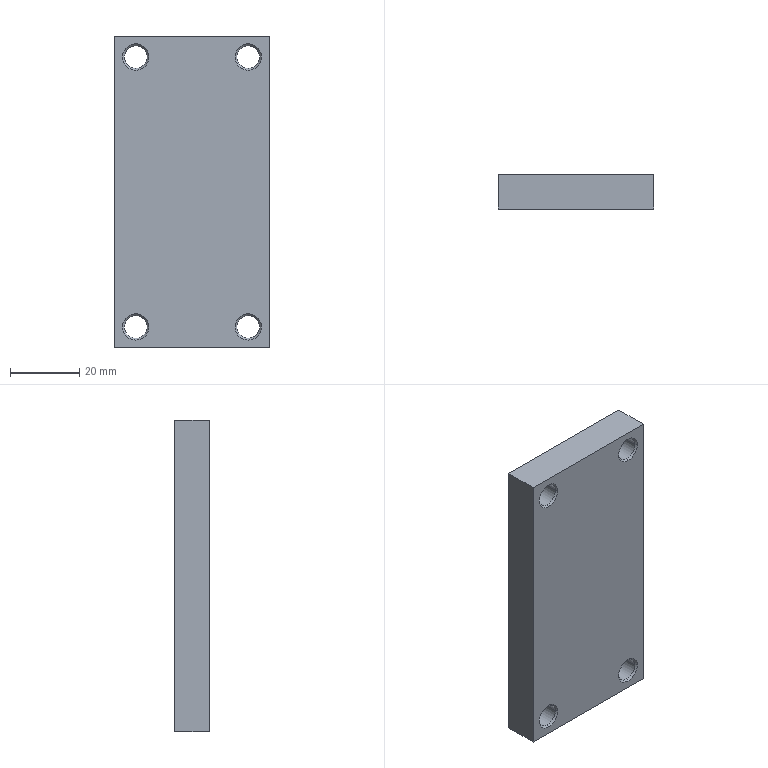Part | STEP file | spacer_5 | 1 solid | 37 faces | box 45 x 10 x 90 mm | volume 39110 mm3 | cone 23 | cylinder 8 | plane 6 | commonest cylinder face diameters 6.6 x8